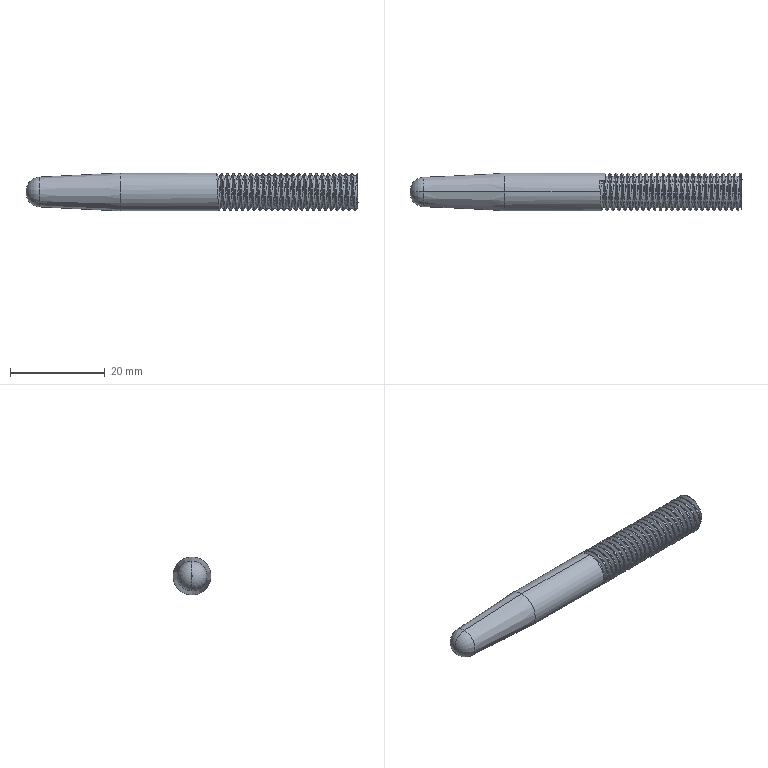Part | SolidWorks | features BaseBody 1 | 1 solid | 107 faces | box 70 x 8 x 8 mm | volume 3017 mm3 | cylinder 98 | plane 3 | torus 2 | cone 2 | spline 2 | commonest cylinder face diameters 6.75 x49 8 x49